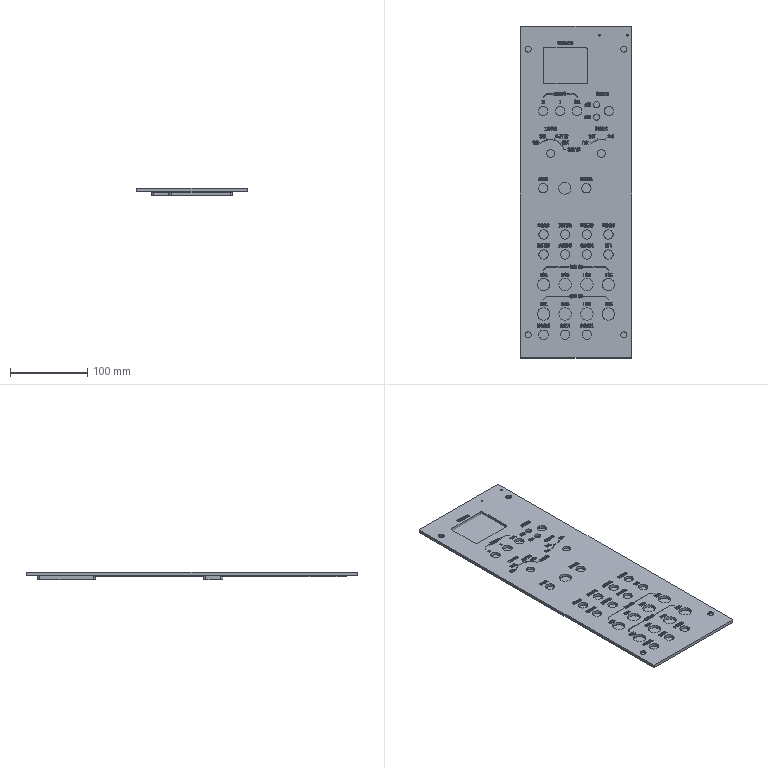NC program | Mastercam | posted with a generic post
Lines 1 to 1000 of 54676:
%
:0001()
(MATERIAL - ALUMINUM MM - 2024)
(T9|10 FEM |H9|XY STOCK TO LEAVE - .15|Z STOCK TO LEAVE - .05)
(T10|10 FEM |H10|XY STOCK TO LEAVE - 0.|Z STOCK TO LEAVE - .05)
(T4|4 FEM |H4)
(T3|3 FEM |H3|XY STOCK TO LEAVE - 0.|Z STOCK TO LEAVE - .15)
(T2|2 FEM |H2|XY STOCK TO LEAVE - .1|Z STOCK TO LEAVE - .1)
(T5|4 CHM |H5|XY STOCK TO LEAVE - 0.|Z STOCK TO LEAVE - .15)
N100 G21
N102 G0 G17 G40 G80 G90 G94 G98
N104 G0 G28 G91 Z0.
N106 G0 G28 X0. Y0.
(10 FEM |TOOL - 9|DIA. OFF. - 9|LEN. - 9|TOOL DIA. - 10.)
N108 T9 M6
N110 G0 G54 G90 X-215. Y79.65 C0. B0. S7000 M3
N112 G43 H9 Z50.
N114 Z1.
N116 G1 Z0. F600.
N118 Y78.65 F3000.
N120 G3 X-214. Y77.65 I1.
N122 G1 X214. Z-.363
N124 G2 X220.15 Y71.5 Z-.371 J-6.15
N126 G1 Y-71.5 Z-.492
N128 G2 X214. Y-77.65 Z-.5 I-6.15
N130 G1 X-214. Z-.863
N132 G2 X-220.15 Y-71.5 Z-.871 J6.15
N134 G1 Y71.5 Z-.992
N136 G2 X-214. Y77.65 Z-1. I6.15
N138 G1 X214. Z-1.363
N140 G2 X220.15 Y71.5 Z-1.371 J-6.15
N142 G1 Y-71.5 Z-1.492
N144 G2 X214. Y-77.65 Z-1.5 I-6.15
N146 G1 X-214. Z-1.863
N148 G2 X-220.15 Y-71.5 Z-1.871 J6.15
N150 G1 Y71.5 Z-1.992
N152 G2 X-214. Y77.65 Z-2. I6.15
N154 G1 X214. Z-2.363
N156 G2 X220.15 Y71.5 Z-2.371 J-6.15
N158 G1 Y-71.5 Z-2.492
N160 G2 X214. Y-77.65 Z-2.5 I-6.15
N162 G1 X-214. Z-2.863
N164 G2 X-220.15 Y-71.5 Z-2.871 J6.15
N166 G1 Y71.5 Z-2.992
N168 G2 X-214. Y77.65 Z-3. I6.15
N170 G1 X214. Z-3.363
N172 G2 X220.15 Y71.5 Z-3.371 J-6.15
N174 G1 Y-71.5 Z-3.492
N176 G2 X214. Y-77.65 Z-3.5 I-6.15
N178 G1 X-214. Z-3.863
N180 G2 X-220.15 Y-71.5 Z-3.871 J6.15
N182 G1 Y71.5 Z-3.992
N184 G2 X-214. Y77.65 Z-4. I6.15
N186 G1 X214. Z-4.363
N188 G2 X220.15 Y71.5 Z-4.371 J-6.15
N190 G1 Y-71.5 Z-4.492
N192 G2 X214. Y-77.65 Z-4.5 I-6.15
N194 G1 X-214. Z-4.863
N196 G2 X-220.15 Y-71.5 Z-4.871 J6.15
N198 G1 Y71.5 Z-4.992
N200 G2 X-214. Y77.65 Z-5. I6.15
N202 G1 X214. Z-5.363
N204 G2 X220.15 Y71.5 Z-5.371 J-6.15
N206 G1 Y-71.5 Z-5.492
N208 G2 X214. Y-77.65 Z-5.5 I-6.15
N210 G1 X-214. Z-5.863
N212 G2 X-220.15 Y-71.5 Z-5.871 J6.15
N214 G1 Y71.5 Z-5.992
N216 G2 X-214. Y77.65 Z-6. I6.15
N218 G1 X214. Z-6.363
N220 G2 X220.15 Y71.5 Z-6.371 J-6.15
N222 G1 Y-71.5 Z-6.492
N224 G2 X214. Y-77.65 Z-6.5 I-6.15
N226 G1 X-214. Z-6.863
N228 G2 X-220.15 Y-71.5 Z-6.871 J6.15
N230 G1 Y71.5 Z-6.992
N232 G2 X-214. Y77.65 Z-7. I6.15
N234 G1 X214. Z-7.363
N236 G2 X220.15 Y71.5 Z-7.371 J-6.15
N238 G1 Y-71.5 Z-7.492
N240 G2 X214. Y-77.65 Z-7.5 I-6.15
N242 G1 X-214. Z-7.863
N244 G2 X-220.15 Y-71.5 Z-7.871 J6.15
N246 G1 Y71.5 Z-7.992
N248 G2 X-214. Y77.65 Z-8. I6.15
N250 G1 X214. Z-8.363
N252 G2 X220.15 Y71.5 Z-8.371 J-6.15
N254 G1 Y-71.5 Z-8.492
N256 G2 X214. Y-77.65 Z-8.5 I-6.15
N258 G1 X-214. Z-8.863
N260 G2 X-220.15 Y-71.5 Z-8.871 J6.15
N262 G1 Y71.5 Z-8.992
N264 G2 X-214. Y77.65 Z-9. I6.15
N266 G1 X214. Z-9.363
N268 G2 X220.15 Y71.5 Z-9.371 J-6.15
N270 G1 Y-71.5 Z-9.492
N272 G2 X214. Y-77.65 Z-9.5 I-6.15
N274 G1 X-214. Z-9.863
N276 G2 X-220.15 Y-71.5 Z-9.871 J6.15
N278 G1 Y22.128 Z-9.95
N280 Y71.5
N282 G2 X-214. Y77.65 I6.15
N284 G1 X214.
N286 G2 X220.15 Y71.5 J-6.15
N288 G1 Y-71.5
N290 G2 X214. Y-77.65 I-6.15
N292 G1 X-214.
N294 G2 X-220.15 Y-71.5 J6.15
N296 G1 Y22.128
N298 G3 X-221.15 Y23.128 I-1.
N300 G1 X-222.15
N302 G0 Z50.
N304 X-113.155 Y-12.874
N306 Z6.87
N308 G1 Z6.37 F600.
N310 Y-12.863 Z6.161 F4000.
N312 Y-12.83 Z5.954
N314 Y-12.776 Z5.752
N316 Y-12.701 Z5.556
N318 Y-12.606 Z5.37
N320 Y-12.492 Z5.194
N322 Y-12.36 Z5.031
N324 Y-12.212 Z4.883
N326 Y-12.049 Z4.752
N328 Y-11.874 Z4.638
N330 Y-11.687 Z4.543
N332 Y-11.492 Z4.468
N334 Y-11.289 Z4.413
N336 Y-11.083 Z4.381
N338 Y-10.874 Z4.37
N340 G2 X-103.155 Y-.874 Z1.6 I10.
N342 G3 X-93.655 Y8.626 Z1.413 J9.5
N344 X-93.893 Y10.74 Z1.386 I-9.5
N346 X-103.155 Y18.126 Z1.225 I-9.262 J-2.114
N348 X-107.277 Y17.186 Z1.171 J-9.5
N350 X-112.656 Y8.626 Z1.037 I4.122 J-8.56
N352 X-110.582 Y2.703 Z.957 I9.501
N354 X-103.155 Y-.874 Z.85 I7.427 J5.923
N356 X-95.728 Y2.703 Z.743 J9.5
N358 X-93.655 Y8.626 Z.663 I-7.427 J5.923
N360 X-99.033 Y17.186 Z.529 I-9.5
N362 X-103.155 Y18.127 Z.475 I-4.122 J-8.56
N364 X-112.417 Y10.74 Z.314 J-9.501
N366 X-112.655 Y8.626 Z.287 I9.262 J-2.114
N368 X-103.155 Y-.874 Z.1 I9.5
N370 G1 X0.
N372 X143.374
N374 Y.873
N376 X-143.374
N378 Y-.874
N380 X-103.155
N382 G2 X-102.148 Y-1.683 J-1.031
N384 G1 X-101.068 Y-6.576
N386 G3 X-100.061 Y-7.385 I1.007 J.222
N388 G1 X0.
N390 X149.885
N392 Y7.385
N394 X-149.885
N396 Y-7.385
N398 X-100.061
N400 G2 X-99.054 Y-8.194 J-1.031
N402 G1 X-97.975 Y-13.087
N404 G3 X-96.967 Y-13.897 I1.008 J.222
N406 G1 X0.
N408 X156.397
N410 Y13.896
N412 X-156.397
N414 Y-13.896
N416 X-96.967 Y-13.897
N418 G2 X-95.96 Y-14.706 J-1.031
N420 G1 X-94.881 Y-19.599
N422 G3 X-93.874 Y-20.408 I1.007 J.222
N424 G1 X0.
N426 X162.908
N428 Y20.408
N430 X-162.908
N432 Y-20.408
N434 X-93.874
N436 G2 X-92.867 Y-21.217 J-1.031
N438 G1 X-91.787 Y-26.11
N440 G3 X-90.78 Y-26.919 I1.007 J.222
N442 G1 X0.
N444 X169.419
N446 Y26.919
N448 X-169.419
N450 Y-26.919
N452 X-90.78
N454 G2 X-89.773 Y-27.728 J-1.032
N456 G1 X-88.693 Y-32.622
N458 G3 X-87.686 Y-33.431 I1.007 J.222
N460 G1 X0.
N462 X175.931
N464 Y33.431
N466 X-175.931
N468 Y-33.431
N470 X-87.686
N472 G2 X-86.679 Y-34.24 J-1.031
N474 G1 X-85.6 Y-39.133
N476 G3 X-84.592 Y-39.942 I1.008 J.222
N478 G1 X0.
N480 X182.442
N482 Y39.942
N484 X-182.442
N486 Y-39.942
N488 X-84.592
N490 G2 X-83.585 Y-40.751 J-1.032
N492 G1 X-82.506 Y-45.645
N494 G3 X-81.499 Y-46.454 I1.007 J.222
N496 G1 X0.
N498 X188.954
N500 Y46.454
N502 X-188.954
N504 Y-46.454
N506 X-81.499
N508 G2 X-80.492 Y-47.263 J-1.031
N510 G1 X-79.412 Y-52.156
N512 G3 X-78.405 Y-52.965 I1.007 J.222
N514 G1 X0.
N516 X195.465
N518 Y52.965
N520 X-195.465
N522 Y-52.965
N524 X-78.405
N526 G2 X-77.398 Y-53.774 J-1.032
N528 G1 X-76.318 Y-58.668
N530 G3 X-75.311 Y-59.477 I1.007 J.223
N532 G1 X0.
N534 X201.977
N536 Y59.477
N538 X-201.977
N540 Y-59.477
N542 X-75.311
N544 G2 X-74.304 Y-60.286 J-1.031
N546 G1 X-73.225 Y-65.179
N548 G3 X-72.218 Y-65.988 I1.007 J.222
N550 G1 X0.
N552 X208.488
N554 Y65.988
N556 X-208.488
N558 Y-65.988
N560 X-72.218
N562 G2 X-71.21 Y-66.797 J-1.031
N564 G1 X-70.131 Y-71.691
N566 G3 X-69.124 Y-72.5 I1.007 J.222
N568 G1 X0.
N570 X214.919
N572 X214.993 Y-72.493
N574 X215. Y-72.419
N576 Y72.419
N578 X214.993 Y72.493
N580 X214.924 Y72.5
N582 X-214.924
N584 X-214.993 Y72.493
N586 X-215. Y72.419
N588 Y-72.419
N590 X-214.993 Y-72.493
N592 X-214.924 Y-72.5
N594 X-69.124
N596 G3 X-67.124 Y-70.5 Z.654 J2.
N598 G1 Y-70.291 Z.665
N600 Y-70.084 Z.698
N602 Y-69.882 Z.752
N604 Y-69.686 Z.827
N606 Y-69.5 Z.922
N608 Y-69.324 Z1.036
N610 Y-69.162 Z1.168
N612 Y-69.014 Z1.316
N614 Y-68.882 Z1.478
N616 Y-68.768 Z1.654
N618 Y-68.673 Z1.84
N620 Y-68.598 Z2.036
N622 Y-68.544 Z2.238
N624 Y-68.511 Z2.445
N626 Y-68.5 Z2.654
N628 Z3.154
N630 G0 Z50.
N632 X-117.326 Y.251
N634 Z2.1
N636 G1 X-117.363 Y.259 Z1.71
N638 X-117.475 Y.282 Z1.335
N640 X-117.656 Y.316 Z.989
N642 X-117.902 Y.356 Z.686
N644 X-118.202 Y.396 Z.437
N646 X-118.546 Y.43 Z.252
N648 X-118.921 Y.453 Z.138
N650 X-119.311 Y.461 Z.1
N652 G3 X-128.811 Y-9.039 Z-.012 J-9.5
N654 X-119.311 Y-18.539 Z-.123 I9.5
N656 X-109.811 Y-9.039 Z-.235 J9.5
N658 X-119.311 Y.461 Z-.346 I-9.5
N660 G1 X-142.961
N662 Y-.461
N664 X-130.05
N666 X-117.139
N668 Y.461
N670 X-119.311
N672 G2 X-120.318 Y1.27 J1.031
N674 G1 X-121.398 Y6.163
N676 G3 X-122.405 Y6.972 I-1.007 J-.222
N678 G1 X-149.472
N680 Y-6.972
N682 X-130.05
N684 X-110.628
N686 Y6.972
N688 X-122.405
N690 G2 X-123.412 Y7.781 J1.031
N692 G1 X-124.491 Y12.675
N694 G3 X-125.498 Y13.484 I-1.007 J-.223
N696 G1 X-155.984
N698 Y-13.484
N700 X-130.05
N702 X-104.116
N704 Y13.484
N706 X-125.498
N708 G2 X-126.505 Y14.293 J1.031
N710 G1 X-127.585 Y19.186
N712 G3 X-128.592 Y19.995 I-1.007 J-.222
N714 G1 X-162.495
N716 Y-19.995
N718 X-130.05
N720 X-97.605
N722 Y19.995
N724 X-128.592
N726 G2 X-129.599 Y20.804 J1.031
N728 G1 X-130.679 Y25.698
N730 G3 X-131.686 Y26.507 I-1.007 J-.223
N732 G1 X-169.007
N734 Y-26.507
N736 X-130.05
N738 X-91.093
N740 Y26.507
N742 X-131.686
N744 G2 X-132.693 Y27.315 J1.031
N746 G1 X-133.773 Y32.191
N748 G3 X-134.78 Y33. I-1.007 J-.223
N750 G1 X-175.5
N752 Y-33.
N754 X-130.05
N756 X-84.219
N758 G2 X-84.6 Y-26.962 I59.019 J6.76
N760 G1 Y33.
N762 X-134.78
N764 G2 X-135.785 Y33.8 J1.031
N766 G1 X-136.868 Y38.52
N768 G3 X-137.873 Y39.321 I-1.005 J-.23
N770 G1 X-181.821
N772 Y-39.321
N774 X-130.05
N776 X-76.396
N778 G2 X-78.266 Y-27.971 I44.681 J13.189
N780 G1 X-78.279 Y39.321
N782 X-137.873
N784 G2 X-138.876 Y40.109 J1.031
N786 G1 X-139.965 Y44.608
N788 G3 X-140.967 Y45.396 I-1.002 J-.243
N790 G1 X-187.897
N792 Y-45.396
N794 X-130.05
N796 X-67.003
N798 G2 X-72.103 Y-29.544 I30.421 J18.532
N800 G1 X-72.203 Y45.396
N802 X-140.967
N804 G2 X-141.964 Y46.165 J1.032
N806 G1 X-143.064 Y50.342
N808 G3 X-144.061 Y51.11 I-.997 J-.263
N810 G1 X-193.611
N812 Y-51.11
N814 X-130.05
N816 X-53.976
N818 G2 X-66.371 Y-29.543 I17.04 J24.138
N820 G1 X-66.406 Y-29.096
N822 X-66.489 Y49.472
N824 X-66.44 Y51.11
N826 X-144.061
N828 G3 X-146.061 Y49.11 Z.208 J-2.
N830 G1 Y48.901 Z.219
N832 Y48.694 Z.251
N834 Y48.492 Z.306
N836 Y48.297 Z.381
N838 Y48.11 Z.476
N840 Y47.935 Z.59
N842 Y47.772 Z.722
N844 Y47.624 Z.87
N846 Y47.492 Z1.032
N848 Y47.378 Z1.208
N850 Y47.283 Z1.394
N852 Y47.208 Z1.59
N854 Y47.154 Z1.792
N856 Y47.121 Z1.999
N858 Y47.11 Z2.208
N860 Z2.708
N862 G0 Z50.
N864 X55.21 Y6.491
N866 Z2.1
N868 G1 X55.202 Y6.454 Z1.71
N870 X55.179 Y6.342 Z1.335
N872 X55.145 Y6.161 Z.989
N874 X55.105 Y5.915 Z.686
N876 X55.065 Y5.615 Z.437
N878 X55.031 Y5.271 Z.252
N880 X55.008 Y4.896 Z.138
N882 X55. Y4.506 Z.1
N884 G3 X64.5 Y-4.994 Z-.012 I9.5
N886 X74. Y4.506 Z-.123 J9.5
N888 X64.5 Y14.006 Z-.235 I-9.5
N890 X55. Y4.506 Z-.346 J-9.5
N892 G1 Y-7.6
N894 Y0.
N896 Y7.6
N898 Y4.506
N900 G2 X54.221 Y3.506 I-1.031
N902 G1 X49.894 Y2.412
N904 G3 X49.116 Y1.412 I.253 J-1.
N906 G1 Y-13.484
N908 X60.884
N910 Y0.
N912 Y13.484
N914 X49.116
N916 Y1.412
N918 G2 X48.307 Y.405 I-1.032
N920 G1 X43.413 Y-.674
N922 G3 X42.604 Y-1.681 I.222 J-1.007
N924 G1 Y-19.996
N926 X67.396
N928 Y0.
N930 Y19.996
N932 X42.604
N934 Y-1.681
N936 G2 X41.795 Y-2.688 I-1.031
N938 G1 X36.902 Y-3.768
N940 G3 X36.093 Y-4.775 I.222 J-1.007
N942 G1 Y-26.507
N944 X73.907
N946 Y0.
N948 Y26.507
N950 X36.093
N952 Y-4.775
N954 G2 X35.284 Y-5.782 I-1.032
N956 G1 X30.408 Y-6.862
N958 G3 X29.6 Y-7.869 I.223 J-1.007
N960 G1 Y-26.962
N962 G2 X29.218 Y-33. I-59.346 J.722
N964 G1 X80.4
N966 Y0.
N968 Y33.
N970 X29.6
N972 Y-7.869
N974 G2 X28.799 Y-8.874 I-1.032
N976 G1 X24.07 Y-9.956
N978 G3 X23.269 Y-10.961 I.23 J-1.005
N980 G1 X23.265 Y-27.971
N982 G2 X21.396 Y-39.321 I-46.164 J1.775
N984 G1 X86.721
N986 Y0.
N988 Y39.321
N990 X23.279
N992 X23.269 Y-10.961
N994 G2 X22.481 Y-11.963 I-1.031
N996 G1 X17.991 Y-13.053
N998 G3 X17.203 Y-14.055 I.243 J-1.002
N1000 G1 Y-26.962
N1002 X17.103 Y-29.544
N1004 G2 X12.003 Y-45.397 I-35.521 J2.68
N1006 G1 X92.797
N1008 Y0.
N1010 Y45.397
N1012 X17.203
N1014 Y-14.055
N1016 G2 X16.435 Y-15.052 I-1.031
N1018 G1 X12.255 Y-16.153
N1020 G3 X11.487 Y-17.15 I.263 J-.997
N1022 G1 X11.489 Y-26.962
N1024 X11.371 Y-29.537
N1026 G2 X-1.022 Y-51.111 I-29.468 J2.582
N1028 G1 X98.56
N1030 X98.511 Y0.
N1032 Y49.472
N1034 X98.56 Y51.111
N1036 X11.44
N1038 X11.469 Y50.498
N1040 X11.487 Y-17.15
N1042 Y-17.151
N1044 G2 X10.763 Y-18.135 I-1.032
N1046 G1 X7.159 Y-19.26
N1048 G3 X6.435 Y-20.244 I.308 J-.984
N1050 G1 Y-26.962
N1052 G2 X5.707 Y-32.886 I-31.826 J.906
N1054 X-10.114 Y-50.125 I-23.745 J5.912
N1056 X-18.018 Y-51.435 I-9.026 J29.955
N1058 G1 X-38.032 Y-51.409
N1060 G2 X-42.896 Y-50.705 I1.805 J29.592
N1062 X-60.976 Y-31.697 I5.915 J23.729
N1064 X-61.435 Y-26.962 I30.697 J5.367
N1066 G1 Y49.472
N1068 G2 X-60.505 Y56.164 I32.778 J-1.146
N1070 G1 X-198.665
N1072 Y-56.164
N1074 X-27.499 Y-56.165
N1076 X104.495
N1078 G2 X103.565 Y-49.472 I31.84 J7.838
N1080 G1 Y49.472
N1082 G2 X104.495 Y56.164 I32.77 J-1.145
N1084 G1 X5.505
N1086 G2 X6.435 Y49.472 I-31.84 J-7.837
N1088 G1 Y-20.244
N1090 G2 X5.647 Y-21.246 I-1.031
N1092 G1 X1.145 Y-22.335
N1094 G3 X.356 Y-23.338 I.242 J-1.003
N1096 G1 Y-26.962
N1098 X.349 Y-27.428
N1100 G2 X-4.176 Y-39.064 I-18.622 J.544
N1102 X-17.229 Y-45.336 I-13.88 J12.168
N1104 G1 X-36.98 Y-45.356
N1106 X-38.694 Y-45.27
N1108 G2 X-49.088 Y-40.803 I1.841 J18.613
N1110 X-55.356 Y-26.962 I12.219 J13.873
N1112 G1 X-55.342 Y50.128
N1114 G2 X-50.209 Y62.244 I18.59 J-.731
N1116 G1 X-204.744
N1118 Y-62.244
N1120 X-27.499
N1122 X114.791
N1124 G2 X109.644 Y-49.472 I13.445 J12.842
N1126 G1 Y49.472
N1128 X109.658 Y50.128
N1130 G2 X114.791 Y62.244 I18.59 J-.731
N1132 G1 X-4.791
N1134 G2 X.356 Y49.472 I-13.446 J-12.842
N1136 G1 Y-23.338
N1138 G2 X-.068 Y-24.171 I-1.031
N1140 G1 X-2.026 Y-25.598
N1142 G3 X-2.45 Y-26.432 I.607 J-.834
N1144 G1 Y-26.962
N1146 G2 X-11.399 Y-41.075 I-15.606 J.001
N1148 X-17.311 Y-42.53 I-7.461 J17.583
N1150 X-27.523 Y-42.67 I-10.212 J372.353
N1152 X-36.98 Y-42.55 J372.493
N1154 X-52.266 Y-29.938 I.007 J15.578
N1156 X-52.55 Y-26.962 I18.925 J3.304
N1158 G1 Y49.472
N1160 G2 X-45.301 Y62.639 I15.63 J-.025
N1162 X-38.471 Y64.972 I8.776 J-14.529
N1164 G1 X-27.499 Y65.05
N1166 X-18.018
N1168 G2 X-2.766 Y52.596 I-.009 J-15.577
N1170 X-2.45 Y49.472 I-19.101 J-3.51
N1172 G1 Y-26.432
N1174 X-2.476 Y-26.664
N1176 X-2.554 Y-26.883
N1178 X-2.679 Y-27.08
N1180 X-2.845 Y-27.244
N1182 X-3.043 Y-27.366
N1184 X-3.264 Y-27.439
N1186 X-9.53 Y-28.793
N1188 G3 X-10.294 Y-29.484 I.218 J-1.008
N1190 G2 X-15.453 Y-34.687 I-7.72 J2.497
N1192 X-18.018 Y-35.1 I-2.645 J8.251
N1194 G1 X-36.98
N1196 G2 X-39.904 Y-34.554 I.036 J8.301
N1198 X-42.428 Y-33.004 I2.878 J7.514
N1200 X-45.048 Y-27.865 I5.411 J5.995
N1202 X-45.1 Y-26.962 I13.307 J1.224
N1204 G1 Y49.472
N1206 Y49.476
N1208 G2 X-43.797 Y53.893 I8.137
N1210 X-40.627 Y56.74 I6.806 J-4.39
N1212 X-37.439 Y57.581 I3.632 J-7.302
N1214 G1 X-36.98 Y57.6
N1216 X-27.499
N1218 X-18.018
N1220 G2 X-15.107 Y57.059 I-.04 J-8.316
N1222 X-12.585 Y55.515 I-2.89 J-7.552
N1224 X-9.953 Y50.368 I-5.41 J-6.013
N1226 X-9.9 Y49.472 I-13.709 J-1.254
N1228 G1 Y-26.962
N1230 Y-26.987
N1232 G2 X-10.294 Y-29.484 I-8.114
N1234 G3 X-10.344 Y-29.801 I.982 J-.317
N1236 X-10.342 Y-29.861 I1.032
N1238 G1 X-8.229 Y-66.578
N1240 G3 X-7.2 Y-67.55 I1.029 J.059
N1242 G1 X210.05
N1244 Y0.
N1246 Y67.55
N1248 X-210.05
N1250 Y-67.55
N1252 X-7.2
N1254 G2 X-6.218 Y-68.266 J-1.031
N1256 G1 X-5.088 Y-71.784
N1258 G3 X-4.106 Y-72.5 I.982 J.315
N1260 G1 X214.919
N1262 X214.993 Y-72.493
N1264 X215. Y-72.419
N1266 Y0.
N1268 Y72.419
N1270 X214.993 Y72.493
N1272 X214.924 Y72.5
N1274 X-214.924
N1276 X-214.993 Y72.493
N1278 X-215. Y72.419
N1280 Y-72.419
N1282 X-214.993 Y-72.493
N1284 X-214.924 Y-72.5
N1286 X-4.106
N1288 G3 X-2.106 Y-70.5 Z.208 J2.
N1290 G1 Y-70.291 Z.219
N1292 Y-70.084 Z.251
N1294 Y-69.882 Z.306
N1296 Y-69.686 Z.381
N1298 Y-69.5 Z.476
N1300 Y-69.324 Z.59
N1302 Y-69.162 Z.722
N1304 Y-69.014 Z.87
N1306 Y-68.882 Z1.032
N1308 Y-68.768 Z1.208
N1310 Y-68.673 Z1.394
N1312 Y-68.598 Z1.59
N1314 Y-68.544 Z1.792
N1316 Y-68.511 Z1.999
N1318 Y-68.5 Z2.208
N1320 Z2.708
N1322 G0 Z50.
N1324 X114.748 Y-50.628
N1326 Z2.1
N1328 G1 X114.756 Y-50.591 Z1.71
N1330 X114.779 Y-50.479 Z1.335
N1332 X114.813 Y-50.298 Z.989
N1334 X114.853 Y-50.052 Z.686
N1336 X114.893 Y-49.752 Z.437
N1338 X114.927 Y-49.408 Z.252
N1340 X114.95 Y-49.033 Z.138
N1342 X114.958 Y-48.643 Z.1
N1344 G3 X105.458 Y-39.144 Z-.012 I-9.5 J-.001
N1346 G1 X105.457
N1348 G3 X95.958 Y-48.644 Z-.123 I.001 J-9.5
N1350 G1 Y-48.645
N1352 G3 X105.458 Y-58.144 Z-.235 I9.5 J.001
N1354 X114.958 Y-48.644 Z-.346 J9.5
N1356 G1 Y-48.643
N1358 X114.95 Y49.472
N1360 Y49.476
N1362 G2 X126.525 Y62.461 I13.072
N1364 G1 X127.451 Y62.534
N1366 X196.998 Y62.55
N1368 G2 X209.79 Y52.07 I-.032 J-13.086
N1370 X210.05 Y49.472 I-15.883 J-2.902
N1372 G1 Y0.
N1374 Y-49.472
N1376 G2 X198.783 Y-62.425 I-13.08 J.001
N1378 G1 X197.769 Y-62.52
N1380 X128.014 Y-62.55
N1382 G2 X115.018 Y-50.756 I.008 J13.067
N1384 G1 X114.958 Y-49.859
N1386 Y-48.643
N1388 G2 X115.673 Y-47.661 I1.031
N1390 G1 X119.185 Y-46.531
N1392 G3 X119.9 Y-45.549 I-.316 J.982
N1394 G1 Y49.472
N1396 Y49.491
N1398 G2 X127.014 Y57.536 I8.106
N1400 X128.014 Y57.6 I1.361 J-13.383
N1402 G1 X196.998
N1404 G2 X205.047 Y50.368 I-.007 J-8.103
N1406 X205.1 Y49.472 I-13.709 J-1.254
N1408 G1 Y0.
N1410 Y-49.472
N1412 Y-49.489
N1414 G2 X198.084 Y-57.524 I-8.11
N1416 G1 X196.998 Y-57.6
N1418 X128.014
N1420 X128.007
N1422 G2 X119.918 Y-49.927 J8.1
N1424 G1 X119.9 Y-49.472
N1426 Y-45.549
N1428 G3 X117.9 Y-43.549 Z.208 I-2.
N1430 G1 X117.691 Z.219
N1432 X117.484 Z.251
N1434 X117.282 Z.306
N1436 X117.087 Z.381
N1438 X116.9 Z.476
N1440 X116.724 Z.59
N1442 X116.562 Z.722
N1444 X116.414 Z.87
N1446 X116.282 Z1.032
N1448 X116.168 Z1.208
N1450 X116.073 Z1.394
N1452 X115.998 Z1.59
N1454 X115.944 Z1.792
N1456 X115.911 Z1.999
N1458 X115.9 Z2.208
N1460 Z2.708
N1462 G0 Z50.
N1464 X54.79 Y-6.492
N1466 Z1.654
N1468 G1 X54.798 Y-6.454 Z1.264
N1470 X54.821 Y-6.343 Z.888
N1472 X54.855 Y-6.161 Z.543
N1474 X54.895 Y-5.915 Z.24
N1476 X54.935 Y-5.615 Z-.009
N1478 X54.969 Y-5.271 Z-.194
N1480 X54.992 Y-4.896 Z-.308
N1482 X55. Y-4.506 Z-.346
N1484 G3 X45.5 Y4.994 Z-.464 I-9.5
N1486 X36. Y-4.506 Z-.582 J-9.5
N1488 X45.5 Y-14.006 Z-.7 I9.5
N1490 X55. Y-4.506 Z-.817 J9.5
N1492 G1 Y0.
N1494 Y7.6
N1496 Y-7.6
N1498 Y-4.506
N1500 G2 X55.779 Y-3.507 I1.031
N1502 G1 X60.106 Y-2.412
N1504 G3 X60.884 Y-1.413 I-.253 J.999
N1506 G1 Y0.
N1508 Y13.484
N1510 X49.116
N1512 Y-13.484
N1514 X60.884
N1516 Y-1.413
N1518 G2 X61.916 Y-.381 I1.032
N1520 X62.07 Y-.393 J-1.032
N1522 G1 X66.21 Y-1.02
N1524 G3 X66.365 Y-1.032 I.155 J1.02
N1526 X67.396 Y0. J1.032
N1528 G1 Y19.996
N1530 X42.604
N1532 Y-19.996
N1534 X67.396
N1536 Y0.
N1538 G2 X68.205 Y1.007 I1.031
N1540 G1 X73.098 Y2.087
N1542 G3 X73.907 Y3.094 I-.222 J1.007
N1544 G1 Y26.507
N1546 X36.093
N1548 Y-26.507
N1550 X73.907
N1552 Y0.
N1554 Y3.094
N1556 G2 X74.716 Y4.101 I1.032
N1558 G1 X79.592 Y5.181
N1560 G3 X80.4 Y6.187 I-.223 J1.006
N1562 G1 Y33.
N1564 X29.6
N1566 Y-26.962
N1568 G2 X29.218 Y-33. I-59.346 J.722
N1570 G1 X80.4
N1572 Y0.
N1574 Y6.187
N1576 G2 X81.201 Y7.193 I1.032
N1578 G1 X85.921 Y8.276
N1580 G3 X86.721 Y9.281 I-.231 J1.005
N1582 G1 Y39.321
N1584 X23.279
N1586 X23.265 Y-27.971
N1588 G2 X21.396 Y-39.321 I-46.164 J1.775
N1590 G1 X86.721
N1592 Y0.
N1594 Y9.281
N1596 G2 X87.51 Y10.283 I1.032
N1598 G1 X92.008 Y11.373
N1600 G3 X92.797 Y12.375 I-.242 J1.002
N1602 G1 Y45.397
N1604 X17.203
N1606 Y-26.962
N1608 X17.103 Y-29.544
N1610 G2 X12.003 Y-45.397 I-35.521 J2.68
N1612 G1 X92.797
N1614 Y0.
N1616 Y12.375
N1618 G2 X93.566 Y13.372 I1.031
N1620 G1 X97.742 Y14.471
N1622 G3 X98.511 Y15.469 I-.262 J.998
N1624 G1 Y49.472
N1626 X98.56 Y51.111
N1628 X11.44
N1630 X11.469 Y50.498
N1632 X11.489 Y-26.962
N1634 X11.371 Y-29.537
N1636 G2 X-1.022 Y-51.111 I-29.468 J2.582
N1638 G1 X98.56
N1640 X98.511 Y0.
N1642 Y15.469
N1644 G3 X96.511 Y17.469 Z-.263 I-2.
N1646 G1 X96.302 Z-.252
N1648 X96.095 Z-.22
N1650 X95.893 Z-.165
N1652 X95.697 Z-.09
N1654 X95.511 Z.005
N1656 X95.335 Z.119
N1658 X95.173 Z.25
N1660 X95.025 Z.398
N1662 X94.893 Z.561
N1664 X94.779 Z.737
N1666 X94.684 Z.923
N1668 X94.609 Z1.119
N1670 X94.555 Z1.321
N1672 X94.522 Z1.528
N1674 X94.511 Z1.737
N1676 Z2.237
N1678 G0 Z50.
N1680 X-118.247 Y.251
N1682 Z1.654
N1684 G1 X-118.285 Y.259 Z1.264
N1686 X-118.397 Y.282 Z.888
N1688 X-118.578 Y.316 Z.543
N1690 X-118.824 Y.356 Z.24
N1692 X-119.124 Y.396 Z-.009
N1694 X-119.468 Y.43 Z-.194
N1696 X-119.843 Y.453 Z-.308
N1698 X-120.233 Y.461 Z-.346
N1700 G3 X-129.733 Y-9.039 Z-.464 J-9.5
N1702 X-120.233 Y-18.539 Z-.582 I9.5
N1704 X-110.733 Y-9.039 Z-.7 J9.5
N1706 X-120.233 Y.461 Z-.817 I-9.5
N1708 G1 X-142.961
N1710 Y-.461
N1712 X-130.05
N1714 X-117.139
N1716 Y.461
N1718 X-120.233
N1720 G2 X-121.24 Y1.27 J1.031
N1722 G1 X-122.319 Y6.163
N1724 G3 X-123.326 Y6.972 I-1.007 J-.222
N1726 G1 X-149.472
N1728 Y-6.972
N1730 X-130.05
N1732 X-110.628
N1734 Y6.972
N1736 X-123.326
N1738 G2 X-124.333 Y7.781 J1.031
N1740 G1 X-125.413 Y12.675
N1742 G3 X-126.42 Y13.484 I-1.007 J-.223
N1744 G1 X-155.984
N1746 Y-13.484
N1748 X-130.05
N1750 X-104.116
N1752 Y13.484
N1754 X-126.42
N1756 G2 X-127.427 Y14.293 J1.031
N1758 G1 X-128.507 Y19.186
N1760 G3 X-129.514 Y19.995 I-1.007 J-.222
N1762 G1 X-162.495
N1764 Y-19.995
N1766 X-130.05
N1768 X-97.605
N1770 Y19.995
N1772 X-129.514
N1774 G2 X-130.521 Y20.804 J1.031
N1776 G1 X-131.601 Y25.698
N1778 G3 X-132.608 Y26.507 I-1.007 J-.223
N1780 G1 X-169.007
N1782 Y-26.507
N1784 X-130.05
N1786 X-91.093
N1788 Y26.507
N1790 X-132.608
N1792 G2 X-133.615 Y27.315 J1.031
N1794 G1 X-134.695 Y32.191
N1796 X-134.77 Y32.41
N1798 X-134.893 Y32.607
N1800 X-135.056 Y32.772
N1802 X-135.252 Y32.895
N1804 X-135.471 Y32.972
N1806 X-135.701 Y33.
N1808 X-175.5
N1810 Y-33.
N1812 X-130.05
N1814 X-84.219
N1816 G2 X-84.6 Y-26.962 I59.019 J6.76
N1818 G1 Y33.
N1820 X-135.701
N1822 G2 X-136.707 Y33.8 J1.031
N1824 G1 X-137.79 Y38.52
N1826 G3 X-138.795 Y39.321 I-1.005 J-.23
N1828 G1 X-181.821
N1830 Y-39.321
N1832 X-130.05
N1834 X-76.396
N1836 G2 X-78.266 Y-27.971 I44.681 J13.189
N1838 G1 X-78.279 Y39.321
N1840 X-138.795
N1842 G2 X-139.797 Y40.109 J1.031
N1844 G1 X-140.887 Y44.608
N1846 G3 X-141.889 Y45.396 I-1.002 J-.243
N1848 G1 X-187.897
N1850 Y-45.396
N1852 X-130.05
N1854 X-67.003
N1856 G2 X-72.103 Y-29.544 I30.421 J18.532
N1858 G1 X-72.203 Y45.396
N1860 X-141.889
N1862 G2 X-142.886 Y46.165 J1.032
N1864 G1 X-143.985 Y50.342
N1866 G3 X-144.983 Y51.11 I-.998 J-.263
N1868 G1 X-193.611
N1870 Y-51.11
N1872 X-130.05
N1874 X-53.976
N1876 G2 X-66.371 Y-29.543 I17.04 J24.138
N1878 G1 X-66.406 Y-29.096
N1880 X-66.489 Y49.472
N1882 X-66.44 Y51.11
N1884 X-144.983
N1886 G2 X-145.967 Y51.834 J1.032
N1888 G1 X-147.092 Y55.44
N1890 G3 X-148.076 Y56.164 I-.984 J-.307
N1892 G1 X-198.665
N1894 Y-56.164
N1896 X-27.499 Y-56.165
N1898 X104.495
N1900 G2 X103.565 Y-49.472 I31.84 J7.838
N1902 G1 Y49.472
N1904 G2 X104.495 Y56.164 I32.77 J-1.145
N1906 G1 X5.505
N1908 G2 X6.435 Y49.472 I-31.84 J-7.837
N1910 G1 Y-26.962
N1912 G2 X5.707 Y-32.886 I-31.826 J.906
N1914 X-10.114 Y-50.125 I-23.745 J5.912
N1916 X-18.018 Y-51.435 I-9.026 J29.955
N1918 G1 X-38.032 Y-51.409
N1920 G2 X-42.896 Y-50.705 I1.805 J29.592
N1922 X-60.976 Y-31.697 I5.915 J23.729
N1924 X-61.435 Y-26.962 I30.697 J5.367
N1926 G1 Y49.472
N1928 G2 X-60.505 Y56.164 I32.778 J-1.146
N1930 G1 X-148.076
N1932 G2 X-149.079 Y56.953 J1.032
N1934 G1 X-150.168 Y61.455
N1936 G3 X-151.17 Y62.244 I-1.002 J-.243
N1938 G1 X-204.744
N1940 Y-62.244
N1942 X-27.499
N1944 X114.791
N1946 G2 X109.644 Y-49.472 I13.445 J12.842
N1948 G1 Y49.472
N1950 X109.658 Y50.128
N1952 G2 X114.791 Y62.244 I18.59 J-.731
N1954 G1 X-4.791
N1956 G2 X.356 Y49.472 I-13.446 J-12.842
N1958 G1 Y-26.962
N1960 X.349 Y-27.428
N1962 G2 X-4.176 Y-39.064 I-18.622 J.544
N1964 X-17.229 Y-45.336 I-13.88 J12.168
N1966 G1 X-36.98 Y-45.356
N1968 X-38.694 Y-45.27
N1970 G2 X-49.088 Y-40.803 I1.841 J18.613
N1972 X-55.356 Y-26.962 I12.219 J13.873
N1974 G1 X-55.342 Y50.128
N1976 G2 X-50.209 Y62.244 I18.59 J-.731
N1978 G1 X-151.17
N1980 G2 X-152.16 Y62.986 J1.031
N1982 G1 X-153.274 Y66.807
N1984 G3 X-154.264 Y67.55 I-.99 J-.288
N1986 G1 X-210.05
N1988 Y-67.55
N1990 X210.05
N1992 Y0.
N1994 Y67.55
N1996 X-154.264
N1998 G2 X-155.246 Y68.266 J1.031
N2000 G1 X-156.376 Y71.784
N2002 G3 X-157.358 Y72.5 I-.982 J-.316
N2004 G1 X-214.924
N2006 X-214.993 Y72.493
N2008 X-215. Y72.419
N2010 Y-72.419
N2012 X-214.993 Y-72.493
N2014 X-214.924 Y-72.5
N2016 X214.919
N2018 X214.993 Y-72.493
N2020 X215. Y-72.419
N2022 Y0.
N2024 Y72.419
N2026 X214.993 Y72.493
N2028 X214.924 Y72.5
N2030 X-157.358
N2032 G3 X-159.358 Y70.5 Z-.263 J-2.
N2034 G1 Y70.291 Z-.252
N2036 Y70.084 Z-.22
N2038 Y69.882 Z-.165
N2040 Y69.686 Z-.09
N2042 Y69.5 Z.005
N2044 Y69.324 Z.119
N2046 Y69.161 Z.25
N2048 Y69.013 Z.398
N2050 Y68.882 Z.561
N2052 Y68.768 Z.737
N2054 Y68.673 Z.923
N2056 Y68.598 Z1.119
N2058 Y68.543 Z1.321
N2060 Y68.511 Z1.528
N2062 Y68.5 Z1.737
N2064 Z2.237
N2066 G0 Z50.
N2068 X-52.337 Y53.587
N2070 Z1.654
N2072 G1 X-52.315 Y53.619 Z1.264
N2074 X-52.252 Y53.714 Z.888
N2076 X-52.152 Y53.869 Z.543
N2078 X-52.023 Y54.082 Z.24